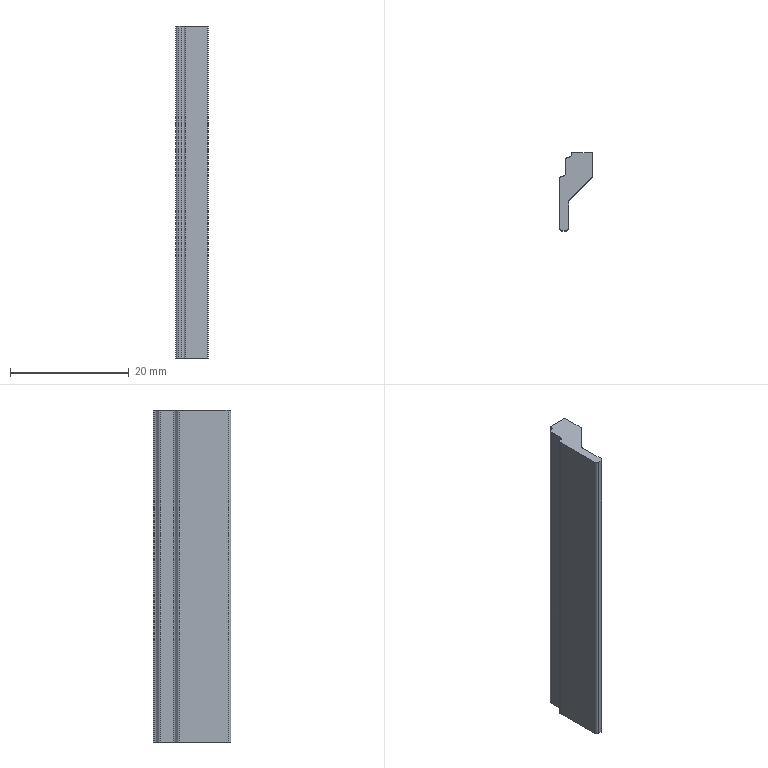Part | NX | features BREP 2 | 2 solids | 36 faces | box 5.515 x 13.15 x 56 mm | volume 4406 mm3 | plane 20 | cylinder 16 | commonest cylinder face diameters 1 x16
STEP:
#1=CARTESIAN_POINT('',(2.758,2.733,-4.));
#2=VERTEX_POINT('',#1);
#3=CARTESIAN_POINT('',(2.758,2.733,52.));
#4=VERTEX_POINT('',#3);
#5=CARTESIAN_POINT('',(2.758,2.733,0.));
#6=DIRECTION('',(0.,0.,1.));
#7=VECTOR('',#6,1000.);
#8=LINE('',#5,#7);
#9=EDGE_CURVE('',#2,#4,#8,.T.);
#10=ORIENTED_EDGE('',*,*,#9,.T.);
#11=CARTESIAN_POINT('',(2.611,2.38,52.));
#12=VERTEX_POINT('',#11);
#13=CARTESIAN_POINT('',(2.258,2.733,52.));
#14=DIRECTION('',(0.,0.,1.));
#15=DIRECTION('',(1.,0.,0.));
#16=AXIS2_PLACEMENT_3D('',#13,#14,#15);
#17=CIRCLE('',#16,0.5);
#18=EDGE_CURVE('',#12,#4,#17,.T.);
#19=ORIENTED_EDGE('',*,*,#18,.F.);
#20=CARTESIAN_POINT('',(2.611,2.38,-4.));
#21=VERTEX_POINT('',#20);
#22=CARTESIAN_POINT('',(2.611,2.38,0.));
#23=DIRECTION('',(0.,0.,1.));
#24=VECTOR('',#23,1000.);
#25=LINE('',#22,#24);
#26=EDGE_CURVE('',#21,#12,#25,.T.);
#27=ORIENTED_EDGE('',*,*,#26,.F.);
#28=CARTESIAN_POINT('',(2.258,2.733,-4.));
#29=DIRECTION('',(0.,0.,1.));
#30=DIRECTION('',(1.,0.,0.));
#31=AXIS2_PLACEMENT_3D('',#28,#29,#30);
#32=CIRCLE('',#31,0.5);
#33=EDGE_CURVE('',#21,#2,#32,.T.);
#34=ORIENTED_EDGE('',*,*,#33,.T.);
#35=EDGE_LOOP('',(#10,#19,#27,#34));
#36=FACE_BOUND('',#35,.T.);
#37=CARTESIAN_POINT('',(2.258,2.733,0.));
#38=DIRECTION('',(0.,0.,1.));
#39=DIRECTION('',(-1.,0.,0.));
#40=AXIS2_PLACEMENT_3D('',#37,#38,#39);
#41=CYLINDRICAL_SURFACE('',#40,0.5);
#42=ADVANCED_FACE('',(#36),#41,.T.);
#43=ORIENTED_EDGE('',*,*,#26,.T.);
#44=CARTESIAN_POINT('',(-1.111,-1.343,52.));
#45=VERTEX_POINT('',#44);
#46=CARTESIAN_POINT('',(2.611,2.38,52.));
#47=DIRECTION('',(0.7071,0.7071,0.));
#48=VECTOR('',#47,1000.);
#49=LINE('',#46,#48);
#50=EDGE_CURVE('',#45,#12,#49,.T.);
#51=ORIENTED_EDGE('',*,*,#50,.F.);
#52=CARTESIAN_POINT('',(-1.111,-1.343,-4.));
#53=VERTEX_POINT('',#52);
#54=CARTESIAN_POINT('',(-1.111,-1.343,0.));
#55=DIRECTION('',(0.,0.,1.));
#56=VECTOR('',#55,1000.);
#57=LINE('',#54,#56);
#58=EDGE_CURVE('',#53,#45,#57,.T.);
#59=ORIENTED_EDGE('',*,*,#58,.F.);
#60=CARTESIAN_POINT('',(2.611,2.38,-4.));
#61=DIRECTION('',(0.7071,0.7071,0.));
#62=VECTOR('',#61,1000.);
#63=LINE('',#60,#62);
#64=EDGE_CURVE('',#53,#21,#63,.T.);
#65=ORIENTED_EDGE('',*,*,#64,.T.);
#66=EDGE_LOOP('',(#43,#51,#59,#65));
#67=FACE_BOUND('',#66,.T.);
#68=CARTESIAN_POINT('',(2.611,2.38,0.));
#69=DIRECTION('',(-0.7071,0.7071,0.));
#70=DIRECTION('',(0.7071,0.7071,0.));
#71=AXIS2_PLACEMENT_3D('',#68,#69,#70);
#72=PLANE('',#71);
#73=ADVANCED_FACE('',(#67),#72,.F.);
#74=ORIENTED_EDGE('',*,*,#58,.T.);
#75=CARTESIAN_POINT('',(-1.258,-1.696,52.));
#76=VERTEX_POINT('',#75);
#77=CARTESIAN_POINT('',(-0.7577,-1.696,52.));
#78=DIRECTION('',(0.,0.,-1.));
#79=DIRECTION('',(1.,0.,0.));
#80=AXIS2_PLACEMENT_3D('',#77,#78,#79);
#81=CIRCLE('',#80,0.5);
#82=EDGE_CURVE('',#76,#45,#81,.T.);
#83=ORIENTED_EDGE('',*,*,#82,.F.);
#84=CARTESIAN_POINT('',(-1.258,-1.696,-4.));
#85=VERTEX_POINT('',#84);
#86=CARTESIAN_POINT('',(-1.258,-1.696,0.));
#87=DIRECTION('',(0.,0.,1.));
#88=VECTOR('',#87,1000.);
#89=LINE('',#86,#88);
#90=EDGE_CURVE('',#85,#76,#89,.T.);
#91=ORIENTED_EDGE('',*,*,#90,.F.);
#92=CARTESIAN_POINT('',(-0.7577,-1.696,-4.));
#93=DIRECTION('',(0.,0.,-1.));
#94=DIRECTION('',(1.,0.,0.));
#95=AXIS2_PLACEMENT_3D('',#92,#93,#94);
#96=CIRCLE('',#95,0.5);
#97=EDGE_CURVE('',#85,#53,#96,.T.);
#98=ORIENTED_EDGE('',*,*,#97,.T.);
#99=EDGE_LOOP('',(#74,#83,#91,#98));
#100=FACE_BOUND('',#99,.T.);
#101=CARTESIAN_POINT('',(-0.7577,-1.696,0.));
#102=DIRECTION('',(0.,0.,1.));
#103=DIRECTION('',(-1.,0.,0.));
#104=AXIS2_PLACEMENT_3D('',#101,#102,#103);
#105=CYLINDRICAL_SURFACE('',#104,0.5);
#106=ADVANCED_FACE('',(#100),#105,.F.);
#107=ORIENTED_EDGE('',*,*,#90,.T.);
#108=CARTESIAN_POINT('',(-1.258,-6.05,52.));
#109=VERTEX_POINT('',#108);
#110=CARTESIAN_POINT('',(-1.258,-8.572,52.));
#111=DIRECTION('',(0.,1.,0.));
#112=VECTOR('',#111,1000.);
#113=LINE('',#110,#112);
#114=EDGE_CURVE('',#109,#76,#113,.T.);
#115=ORIENTED_EDGE('',*,*,#114,.F.);
#116=CARTESIAN_POINT('',(-1.258,-6.05,-4.));
#117=VERTEX_POINT('',#116);
#118=CARTESIAN_POINT('',(-1.258,-6.05,0.));
#119=DIRECTION('',(0.,0.,1.));
#120=VECTOR('',#119,1000.);
#121=LINE('',#118,#120);
#122=EDGE_CURVE('',#117,#109,#121,.T.);
#123=ORIENTED_EDGE('',*,*,#122,.F.);
#124=CARTESIAN_POINT('',(-1.258,-8.572,-4.));
#125=DIRECTION('',(0.,1.,0.));
#126=VECTOR('',#125,1000.);
#127=LINE('',#124,#126);
#128=EDGE_CURVE('',#117,#85,#127,.T.);
#129=ORIENTED_EDGE('',*,*,#128,.T.);
#130=EDGE_LOOP('',(#107,#115,#123,#129));
#131=FACE_BOUND('',#130,.T.);
#132=CARTESIAN_POINT('',(-1.258,-1.696,0.));
#133=DIRECTION('',(-1.,0.,0.));
#134=DIRECTION('',(0.,1.,0.));
#135=AXIS2_PLACEMENT_3D('',#132,#133,#134);
#136=PLANE('',#135);
#137=ADVANCED_FACE('',(#131),#136,.F.);
#138=ORIENTED_EDGE('',*,*,#122,.T.);
#139=CARTESIAN_POINT('',(-1.758,-6.55,52.));
#140=VERTEX_POINT('',#139);
#141=CARTESIAN_POINT('',(-1.758,-6.05,52.));
#142=DIRECTION('',(0.,0.,1.));
#143=DIRECTION('',(1.,0.,0.));
#144=AXIS2_PLACEMENT_3D('',#141,#142,#143);
#145=CIRCLE('',#144,0.5);
#146=EDGE_CURVE('',#140,#109,#145,.T.);
#147=ORIENTED_EDGE('',*,*,#146,.F.);
#148=CARTESIAN_POINT('',(-1.758,-6.55,-4.));
#149=VERTEX_POINT('',#148);
#150=CARTESIAN_POINT('',(-1.758,-6.55,0.));
#151=DIRECTION('',(0.,0.,1.));
#152=VECTOR('',#151,1000.);
#153=LINE('',#150,#152);
#154=EDGE_CURVE('',#149,#140,#153,.T.);
#155=ORIENTED_EDGE('',*,*,#154,.F.);
#156=CARTESIAN_POINT('',(-1.758,-6.05,-4.));
#157=DIRECTION('',(0.,0.,1.));
#158=DIRECTION('',(1.,0.,0.));
#159=AXIS2_PLACEMENT_3D('',#156,#157,#158);
#160=CIRCLE('',#159,0.5);
#161=EDGE_CURVE('',#149,#117,#160,.T.);
#162=ORIENTED_EDGE('',*,*,#161,.T.);
#163=EDGE_LOOP('',(#138,#147,#155,#162));
#164=FACE_BOUND('',#163,.T.);
#165=CARTESIAN_POINT('',(-1.758,-6.05,0.));
#166=DIRECTION('',(0.,0.,1.));
#167=DIRECTION('',(-1.,0.,0.));
#168=AXIS2_PLACEMENT_3D('',#165,#166,#167);
#169=CYLINDRICAL_SURFACE('',#168,0.5);
#170=ADVANCED_FACE('',(#164),#169,.T.);
#171=ORIENTED_EDGE('',*,*,#154,.T.);
#172=CARTESIAN_POINT('',(-2.258,-6.55,52.));
#173=VERTEX_POINT('',#172);
#174=CARTESIAN_POINT('',(6.216,-6.55,52.));
#175=DIRECTION('',(1.,0.,0.));
#176=VECTOR('',#175,1000.);
#177=LINE('',#174,#176);
#178=EDGE_CURVE('',#173,#140,#177,.T.);
#179=ORIENTED_EDGE('',*,*,#178,.F.);
#180=CARTESIAN_POINT('',(-2.258,-6.55,-4.));
#181=VERTEX_POINT('',#180);
#182=CARTESIAN_POINT('',(-2.258,-6.55,0.));
#183=DIRECTION('',(0.,0.,1.));
#184=VECTOR('',#183,1000.);
#185=LINE('',#182,#184);
#186=EDGE_CURVE('',#181,#173,#185,.T.);
#187=ORIENTED_EDGE('',*,*,#186,.F.);
#188=CARTESIAN_POINT('',(6.216,-6.55,-4.));
#189=DIRECTION('',(1.,0.,0.));
#190=VECTOR('',#189,1000.);
#191=LINE('',#188,#190);
#192=EDGE_CURVE('',#181,#149,#191,.T.);
#193=ORIENTED_EDGE('',*,*,#192,.T.);
#194=EDGE_LOOP('',(#171,#179,#187,#193));
#195=FACE_BOUND('',#194,.T.);
#196=CARTESIAN_POINT('',(-1.758,-6.55,0.));
#197=DIRECTION('',(0.,1.,0.));
#198=DIRECTION('',(1.,0.,0.));
#199=AXIS2_PLACEMENT_3D('',#196,#197,#198);
#200=PLANE('',#199);
#201=ADVANCED_FACE('',(#195),#200,.F.);
#202=ORIENTED_EDGE('',*,*,#186,.T.);
#203=CARTESIAN_POINT('',(-2.758,-6.05,52.));
#204=VERTEX_POINT('',#203);
#205=CARTESIAN_POINT('',(-2.258,-6.05,52.));
#206=DIRECTION('',(0.,0.,1.));
#207=DIRECTION('',(1.,0.,0.));
#208=AXIS2_PLACEMENT_3D('',#205,#206,#207);
#209=CIRCLE('',#208,0.5);
#210=EDGE_CURVE('',#204,#173,#209,.T.);
#211=ORIENTED_EDGE('',*,*,#210,.F.);
#212=CARTESIAN_POINT('',(-2.758,-6.05,-4.));
#213=VERTEX_POINT('',#212);
#214=CARTESIAN_POINT('',(-2.758,-6.05,0.));
#215=DIRECTION('',(0.,0.,1.));
#216=VECTOR('',#215,1000.);
#217=LINE('',#214,#216);
#218=EDGE_CURVE('',#213,#204,#217,.T.);
#219=ORIENTED_EDGE('',*,*,#218,.F.);
#220=CARTESIAN_POINT('',(-2.258,-6.05,-4.));
#221=DIRECTION('',(0.,0.,1.));
#222=DIRECTION('',(1.,0.,0.));
#223=AXIS2_PLACEMENT_3D('',#220,#221,#222);
#224=CIRCLE('',#223,0.5);
#225=EDGE_CURVE('',#213,#181,#224,.T.);
#226=ORIENTED_EDGE('',*,*,#225,.T.);
#227=EDGE_LOOP('',(#202,#211,#219,#226));
#228=FACE_BOUND('',#227,.T.);
#229=CARTESIAN_POINT('',(-2.258,-6.05,0.));
#230=DIRECTION('',(0.,0.,1.));
#231=DIRECTION('',(-1.,0.,0.));
#232=AXIS2_PLACEMENT_3D('',#229,#230,#231);
#233=CYLINDRICAL_SURFACE('',#232,0.5);
#234=ADVANCED_FACE('',(#228),#233,.T.);
#235=ORIENTED_EDGE('',*,*,#218,.T.);
#236=CARTESIAN_POINT('',(-2.758,2.15,52.));
#237=VERTEX_POINT('',#236);
#238=CARTESIAN_POINT('',(-2.758,-8.572,52.));
#239=DIRECTION('',(0.,-1.,0.));
#240=VECTOR('',#239,1000.);
#241=LINE('',#238,#240);
#242=EDGE_CURVE('',#237,#204,#241,.T.);
#243=ORIENTED_EDGE('',*,*,#242,.F.);
#244=CARTESIAN_POINT('',(-2.758,2.15,-4.));
#245=VERTEX_POINT('',#244);
#246=CARTESIAN_POINT('',(-2.758,2.15,0.));
#247=DIRECTION('',(0.,0.,1.));
#248=VECTOR('',#247,1000.);
#249=LINE('',#246,#248);
#250=EDGE_CURVE('',#245,#237,#249,.T.);
#251=ORIENTED_EDGE('',*,*,#250,.F.);
#252=CARTESIAN_POINT('',(-2.758,-8.572,-4.));
#253=DIRECTION('',(0.,-1.,0.));
#254=VECTOR('',#253,1000.);
#255=LINE('',#252,#254);
#256=EDGE_CURVE('',#245,#213,#255,.T.);
#257=ORIENTED_EDGE('',*,*,#256,.T.);
#258=EDGE_LOOP('',(#235,#243,#251,#257));
#259=FACE_BOUND('',#258,.T.);
#260=CARTESIAN_POINT('',(-2.758,-6.05,0.));
#261=DIRECTION('',(1.,0.,0.));
#262=DIRECTION('',(0.,-1.,0.));
#263=AXIS2_PLACEMENT_3D('',#260,#261,#262);
#264=PLANE('',#263);
#265=ADVANCED_FACE('',(#259),#264,.F.);
#266=ORIENTED_EDGE('',*,*,#250,.T.);
#267=CARTESIAN_POINT('',(-2.258,2.65,52.));
#268=VERTEX_POINT('',#267);
#269=CARTESIAN_POINT('',(-2.258,2.15,52.));
#270=DIRECTION('',(0.,0.,1.));
#271=DIRECTION('',(1.,0.,0.));
#272=AXIS2_PLACEMENT_3D('',#269,#270,#271);
#273=CIRCLE('',#272,0.5);
#274=EDGE_CURVE('',#268,#237,#273,.T.);
#275=ORIENTED_EDGE('',*,*,#274,.F.);
#276=CARTESIAN_POINT('',(-2.258,2.65,-4.));
#277=VERTEX_POINT('',#276);
#278=CARTESIAN_POINT('',(-2.258,2.65,0.));
#279=DIRECTION('',(0.,0.,1.));
#280=VECTOR('',#279,1000.);
#281=LINE('',#278,#280);
#282=EDGE_CURVE('',#277,#268,#281,.T.);
#283=ORIENTED_EDGE('',*,*,#282,.F.);
#284=CARTESIAN_POINT('',(-2.258,2.15,-4.));
#285=DIRECTION('',(0.,0.,1.));
#286=DIRECTION('',(1.,0.,0.));
#287=AXIS2_PLACEMENT_3D('',#284,#285,#286);
#288=CIRCLE('',#287,0.5);
#289=EDGE_CURVE('',#277,#245,#288,.T.);
#290=ORIENTED_EDGE('',*,*,#289,.T.);
#291=EDGE_LOOP('',(#266,#275,#283,#290));
#292=FACE_BOUND('',#291,.T.);
#293=CARTESIAN_POINT('',(-2.258,2.15,0.));
#294=DIRECTION('',(0.,0.,1.));
#295=DIRECTION('',(-1.,0.,0.));
#296=AXIS2_PLACEMENT_3D('',#293,#294,#295);
#297=CYLINDRICAL_SURFACE('',#296,0.5);
#298=ADVANCED_FACE('',(#292),#297,.T.);
#299=ORIENTED_EDGE('',*,*,#282,.T.);
#300=CARTESIAN_POINT('',(-1.758,3.15,52.));
#301=VERTEX_POINT('',#300);
#302=CARTESIAN_POINT('',(-2.258,3.15,52.));
#303=DIRECTION('',(0.,0.,-1.));
#304=DIRECTION('',(1.,0.,0.));
#305=AXIS2_PLACEMENT_3D('',#302,#303,#304);
#306=CIRCLE('',#305,0.5);
#307=EDGE_CURVE('',#301,#268,#306,.T.);
#308=ORIENTED_EDGE('',*,*,#307,.F.);
#309=CARTESIAN_POINT('',(-1.758,3.15,-4.));
#310=VERTEX_POINT('',#309);
#311=CARTESIAN_POINT('',(-1.758,3.15,0.));
#312=DIRECTION('',(0.,0.,1.));
#313=VECTOR('',#312,1000.);
#314=LINE('',#311,#313);
#315=EDGE_CURVE('',#310,#301,#314,.T.);
#316=ORIENTED_EDGE('',*,*,#315,.F.);
#317=CARTESIAN_POINT('',(-2.258,3.15,-4.));
#318=DIRECTION('',(0.,0.,-1.));
#319=DIRECTION('',(1.,0.,0.));
#320=AXIS2_PLACEMENT_3D('',#317,#318,#319);
#321=CIRCLE('',#320,0.5);
#322=EDGE_CURVE('',#310,#277,#321,.T.);
#323=ORIENTED_EDGE('',*,*,#322,.T.);
#324=EDGE_LOOP('',(#299,#308,#316,#323));
#325=FACE_BOUND('',#324,.T.);
#326=CARTESIAN_POINT('',(-2.258,3.15,0.));
#327=DIRECTION('',(0.,0.,1.));
#328=DIRECTION('',(-1.,0.,0.));
#329=AXIS2_PLACEMENT_3D('',#326,#327,#328);
#330=CYLINDRICAL_SURFACE('',#329,0.5);
#331=ADVANCED_FACE('',(#325),#330,.F.);
#332=ORIENTED_EDGE('',*,*,#315,.T.);
#333=CARTESIAN_POINT('',(-1.758,5.35,52.));
#334=VERTEX_POINT('',#333);
#335=CARTESIAN_POINT('',(-1.758,-8.572,52.));
#336=DIRECTION('',(0.,-1.,0.));
#337=VECTOR('',#336,1000.);
#338=LINE('',#335,#337);
#339=EDGE_CURVE('',#334,#301,#338,.T.);
#340=ORIENTED_EDGE('',*,*,#339,.F.);
#341=CARTESIAN_POINT('',(-1.758,5.35,-4.));
#342=VERTEX_POINT('',#341);
#343=CARTESIAN_POINT('',(-1.758,5.35,0.));
#344=DIRECTION('',(0.,0.,1.));
#345=VECTOR('',#344,1000.);
#346=LINE('',#343,#345);
#347=EDGE_CURVE('',#342,#334,#346,.T.);
#348=ORIENTED_EDGE('',*,*,#347,.F.);
#349=CARTESIAN_POINT('',(-1.758,-8.572,-4.));
#350=DIRECTION('',(0.,-1.,0.));
#351=VECTOR('',#350,1000.);
#352=LINE('',#349,#351);
#353=EDGE_CURVE('',#342,#310,#352,.T.);
#354=ORIENTED_EDGE('',*,*,#353,.T.);
#355=EDGE_LOOP('',(#332,#340,#348,#354));
#356=FACE_BOUND('',#355,.T.);
#357=CARTESIAN_POINT('',(-1.758,3.15,0.));
#358=DIRECTION('',(1.,0.,0.));
#359=DIRECTION('',(0.,-1.,0.));
#360=AXIS2_PLACEMENT_3D('',#357,#358,#359);
#361=PLANE('',#360);
#362=ADVANCED_FACE('',(#356),#361,.F.);
#363=ORIENTED_EDGE('',*,*,#347,.T.);
#364=CARTESIAN_POINT('',(-1.258,5.85,52.));
#365=VERTEX_POINT('',#364);
#366=CARTESIAN_POINT('',(-1.258,5.35,52.));
#367=DIRECTION('',(0.,0.,1.));
#368=DIRECTION('',(1.,0.,0.));
#369=AXIS2_PLACEMENT_3D('',#366,#367,#368);
#370=CIRCLE('',#369,0.5);
#371=EDGE_CURVE('',#365,#334,#370,.T.);
#372=ORIENTED_EDGE('',*,*,#371,.F.);
#373=CARTESIAN_POINT('',(-1.258,5.85,-4.));
#374=VERTEX_POINT('',#373);
#375=CARTESIAN_POINT('',(-1.258,5.85,0.));
#376=DIRECTION('',(0.,0.,1.));
#377=VECTOR('',#376,1000.);
#378=LINE('',#375,#377);
#379=EDGE_CURVE('',#374,#365,#378,.T.);
#380=ORIENTED_EDGE('',*,*,#379,.F.);
#381=CARTESIAN_POINT('',(-1.258,5.35,-4.));
#382=DIRECTION('',(0.,0.,1.));
#383=DIRECTION('',(1.,0.,0.));
#384=AXIS2_PLACEMENT_3D('',#381,#382,#383);
#385=CIRCLE('',#384,0.5);
#386=EDGE_CURVE('',#374,#342,#385,.T.);
#387=ORIENTED_EDGE('',*,*,#386,.T.);
#388=EDGE_LOOP('',(#363,#372,#380,#387));
#389=FACE_BOUND('',#388,.T.);
#390=CARTESIAN_POINT('',(-1.258,5.35,0.));
#391=DIRECTION('',(0.,0.,1.));
#392=DIRECTION('',(-1.,0.,0.));
#393=AXIS2_PLACEMENT_3D('',#390,#391,#392);
#394=CYLINDRICAL_SURFACE('',#393,0.5);
#395=ADVANCED_FACE('',(#389),#394,.T.);
#396=ORIENTED_EDGE('',*,*,#379,.T.);
#397=CARTESIAN_POINT('',(-0.7577,6.35,52.));
#398=VERTEX_POINT('',#397);
#399=CARTESIAN_POINT('',(-1.258,6.35,52.));
#400=DIRECTION('',(0.,0.,-1.));
#401=DIRECTION('',(1.,0.,0.));
#402=AXIS2_PLACEMENT_3D('',#399,#400,#401);
#403=CIRCLE('',#402,0.5);
#404=EDGE_CURVE('',#398,#365,#403,.T.);
#405=ORIENTED_EDGE('',*,*,#404,.F.);
#406=CARTESIAN_POINT('',(-0.7577,6.35,-4.));
#407=VERTEX_POINT('',#406);
#408=CARTESIAN_POINT('',(-0.7577,6.35,0.));
#409=DIRECTION('',(0.,0.,1.));
#410=VECTOR('',#409,1000.);
#411=LINE('',#408,#410);
#412=EDGE_CURVE('',#407,#398,#411,.T.);
#413=ORIENTED_EDGE('',*,*,#412,.F.);
#414=CARTESIAN_POINT('',(-1.258,6.35,-4.));
#415=DIRECTION('',(0.,0.,-1.));
#416=DIRECTION('',(1.,0.,0.));
#417=AXIS2_PLACEMENT_3D('',#414,#415,#416);
#418=CIRCLE('',#417,0.5);
#419=EDGE_CURVE('',#407,#374,#418,.T.);
#420=ORIENTED_EDGE('',*,*,#419,.T.);
#421=EDGE_LOOP('',(#396,#405,#413,#420));
#422=FACE_BOUND('',#421,.T.);
#423=CARTESIAN_POINT('',(-1.258,6.35,0.));
#424=DIRECTION('',(0.,0.,1.));
#425=DIRECTION('',(-1.,0.,0.));
#426=AXIS2_PLACEMENT_3D('',#423,#424,#425);
#427=CYLINDRICAL_SURFACE('',#426,0.5);
#428=ADVANCED_FACE('',(#422),#427,.F.);
#429=ORIENTED_EDGE('',*,*,#412,.T.);
#430=CARTESIAN_POINT('',(-0.7577,6.6,52.));
#431=VERTEX_POINT('',#430);
#432=CARTESIAN_POINT('',(-0.7577,-8.572,52.));
#433=DIRECTION('',(0.,-1.,0.));
#434=VECTOR('',#433,1000.);
#435=LINE('',#432,#434);
#436=EDGE_CURVE('',#431,#398,#435,.T.);
#437=ORIENTED_EDGE('',*,*,#436,.F.);
#438=CARTESIAN_POINT('',(-0.7577,6.6,-4.));
#439=VERTEX_POINT('',#438);
#440=CARTESIAN_POINT('',(-0.7577,6.6,0.));
#441=DIRECTION('',(0.,0.,1.));
#442=VECTOR('',#441,1000.);
#443=LINE('',#440,#442);
#444=EDGE_CURVE('',#439,#431,#443,.T.);
#445=ORIENTED_EDGE('',*,*,#444,.F.);
#446=CARTESIAN_POINT('',(-0.7577,-8.572,-4.));
#447=DIRECTION('',(0.,-1.,0.));
#448=VECTOR('',#447,1000.);
#449=LINE('',#446,#448);
#450=EDGE_CURVE('',#439,#407,#449,.T.);
#451=ORIENTED_EDGE('',*,*,#450,.T.);
#452=EDGE_LOOP('',(#429,#437,#445,#451));
#453=FACE_BOUND('',#452,.T.);
#454=CARTESIAN_POINT('',(-0.7577,6.35,0.));
#455=DIRECTION('',(1.,0.,0.));
#456=DIRECTION('',(0.,-1.,0.));
#457=AXIS2_PLACEMENT_3D('',#454,#455,#456);
#458=PLANE('',#457);
#459=ADVANCED_FACE('',(#453),#458,.F.);
#460=ORIENTED_EDGE('',*,*,#444,.T.);
#461=CARTESIAN_POINT('',(2.758,6.6,52.));
#462=VERTEX_POINT('',#461);
#463=CARTESIAN_POINT('',(6.216,6.6,52.));
#464=DIRECTION('',(-1.,0.,0.));
#465=VECTOR('',#464,1000.);
#466=LINE('',#463,#465);
#467=EDGE_CURVE('',#462,#431,#466,.T.);
#468=ORIENTED_EDGE('',*,*,#467,.F.);
#469=CARTESIAN_POINT('',(2.758,6.6,-4.));
#470=VERTEX_POINT('',#469);
#471=CARTESIAN_POINT('',(2.758,6.6,0.));
#472=DIRECTION('',(0.,0.,1.));
#473=VECTOR('',#472,1000.);
#474=LINE('',#471,#473);
#475=EDGE_CURVE('',#470,#462,#474,.T.);
#476=ORIENTED_EDGE('',*,*,#475,.F.);
#477=CARTESIAN_POINT('',(6.216,6.6,-4.));
#478=DIRECTION('',(-1.,0.,0.));
#479=VECTOR('',#478,1000.);
#480=LINE('',#477,#479);
#481=EDGE_CURVE('',#470,#439,#480,.T.);
#482=ORIENTED_EDGE('',*,*,#481,.T.);
#483=EDGE_LOOP('',(#460,#468,#476,#482));
#484=FACE_BOUND('',#483,.T.);
#485=CARTESIAN_POINT('',(6.216,6.6,0.));
#486=DIRECTION('',(0.,-1.,0.));
#487=DIRECTION('',(-1.,0.,0.));
#488=AXIS2_PLACEMENT_3D('',#485,#486,#487);
#489=PLANE('',#488);
#490=ADVANCED_FACE('',(#484),#489,.F.);
#491=CARTESIAN_POINT('',(2.758,-8.572,-4.));
#492=DIRECTION('',(0.,1.,0.));
#493=VECTOR('',#492,1000.);
#494=LINE('',#491,#493);
#495=EDGE_CURVE('',#2,#470,#494,.T.);
#496=ORIENTED_EDGE('',*,*,#495,.T.);
#497=ORIENTED_EDGE('',*,*,#475,.T.);
#498=CARTESIAN_POINT('',(2.758,-8.572,52.));
#499=DIRECTION('',(0.,1.,0.));
#500=VECTOR('',#499,1000.);
#501=LINE('',#498,#500);
#502=EDGE_CURVE('',#4,#462,#501,.T.);
#503=ORIENTED_EDGE('',*,*,#502,.F.);
#504=ORIENTED_EDGE('',*,*,#9,.F.);
#505=EDGE_LOOP('',(#496,#497,#503,#504));
#506=FACE_BOUND('',#505,.T.);
#507=CARTESIAN_POINT('',(2.758,8.726,0.));
#508=DIRECTION('',(-1.,0.,0.));
#509=DIRECTION('',(0.,1.,0.));
#510=AXIS2_PLACEMENT_3D('',#507,#508,#509);
#511=PLANE('',#510);
#512=ADVANCED_FACE('',(#506),#511,.F.);
#513=ORIENTED_EDGE('',*,*,#467,.T.);
#514=ORIENTED_EDGE('',*,*,#436,.T.);
#515=ORIENTED_EDGE('',*,*,#404,.T.);
#516=ORIENTED_EDGE('',*,*,#371,.T.);
#517=ORIENTED_EDGE('',*,*,#339,.T.);
#518=ORIENTED_EDGE('',*,*,#307,.T.);
#519=ORIENTED_EDGE('',*,*,#274,.T.);
#520=ORIENTED_EDGE('',*,*,#242,.T.);
#521=ORIENTED_EDGE('',*,*,#210,.T.);
#522=ORIENTED_EDGE('',*,*,#178,.T.);
#523=ORIENTED_EDGE('',*,*,#146,.T.);
#524=ORIENTED_EDGE('',*,*,#114,.T.);
#525=ORIENTED_EDGE('',*,*,#82,.T.);
#526=ORIENTED_EDGE('',*,*,#50,.T.);
#527=ORIENTED_EDGE('',*,*,#18,.T.);
#528=ORIENTED_EDGE('',*,*,#502,.T.);
#529=EDGE_LOOP('',(#513,#514,#515,#516,#517,#518,#519,#520,#521,#522,#523,#524,#525,#526,#527,#528));
#530=FACE_BOUND('',#529,.T.);
#531=CARTESIAN_POINT('',(6.216,-8.572,52.));
#532=DIRECTION('',(0.,0.,1.));
#533=DIRECTION('',(-1.,0.,0.));
#534=AXIS2_PLACEMENT_3D('',#531,#532,#533);
#535=PLANE('',#534);
#536=ADVANCED_FACE('',(#530),#535,.T.);
#537=ORIENTED_EDGE('',*,*,#481,.F.);
#538=ORIENTED_EDGE('',*,*,#495,.F.);
#539=ORIENTED_EDGE('',*,*,#33,.F.);
#540=ORIENTED_EDGE('',*,*,#64,.F.);
#541=ORIENTED_EDGE('',*,*,#97,.F.);
#542=ORIENTED_EDGE('',*,*,#128,.F.);
#543=ORIENTED_EDGE('',*,*,#161,.F.);
#544=ORIENTED_EDGE('',*,*,#192,.F.);
#545=ORIENTED_EDGE('',*,*,#225,.F.);
#546=ORIENTED_EDGE('',*,*,#256,.F.);
#547=ORIENTED_EDGE('',*,*,#289,.F.);
#548=ORIENTED_EDGE('',*,*,#322,.F.);
#549=ORIENTED_EDGE('',*,*,#353,.F.);
#550=ORIENTED_EDGE('',*,*,#386,.F.);
#551=ORIENTED_EDGE('',*,*,#419,.F.);
#552=ORIENTED_EDGE('',*,*,#450,.F.);
#553=EDGE_LOOP('',(#537,#538,#539,#540,#541,#542,#543,#544,#545,#546,#547,#548,#549,#550,#551,#552));
#554=FACE_BOUND('',#553,.T.);
#555=CARTESIAN_POINT('',(6.216,-8.572,-4.));
#556=DIRECTION('',(0.,0.,1.));
#557=DIRECTION('',(-1.,0.,0.));
#558=AXIS2_PLACEMENT_3D('',#555,#556,#557);
#559=PLANE('',#558);
#560=ADVANCED_FACE('',(#554),#559,.F.);
#561=CLOSED_SHELL('',(#42,#73,#106,#137,#170,#201,#234,#265,#298,#331,#362,#395,#428,#459,#490,#512,#536,#560));
#562=MANIFOLD_SOLID_BREP('',#561);
#563=CARTESIAN_POINT('',(2.758,2.733,-4.));
#564=VERTEX_POINT('',#563);
#565=CARTESIAN_POINT('',(2.758,2.733,52.));
#566=VERTEX_POINT('',#565);
#567=CARTESIAN_POINT('',(2.758,2.733,0.));
#568=DIRECTION('',(0.,0.,1.));
#569=VECTOR('',#568,1000.);
#570=LINE('',#567,#569);
#571=EDGE_CURVE('',#564,#566,#570,.T.);
#572=ORIENTED_EDGE('',*,*,#571,.T.);
#573=CARTESIAN_POINT('',(2.611,2.38,52.));
#574=VERTEX_POINT('',#573);
#575=CARTESIAN_POINT('',(2.258,2.733,52.));
#576=DIRECTION('',(0.,0.,1.));
#577=DIRECTION('',(1.,0.,0.));
#578=AXIS2_PLACEMENT_3D('',#575,#576,#577);
#579=CIRCLE('',#578,0.5);
#580=EDGE_CURVE('',#574,#566,#579,.T.);
#581=ORIENTED_EDGE('',*,*,#580,.F.);
#582=CARTESIAN_POINT('',(2.611,2.38,-4.));
#583=VERTEX_POINT('',#582);
#584=CARTESIAN_POINT('',(2.611,2.38,0.));
#585=DIRECTION('',(0.,0.,1.));
#586=VECTOR('',#585,1000.);
#587=LINE('',#584,#586);
#588=EDGE_CURVE('',#583,#574,#587,.T.);
#589=ORIENTED_EDGE('',*,*,#588,.F.);
#590=CARTESIAN_POINT('',(2.258,2.733,-4.));
#591=DIRECTION('',(0.,0.,1.));
#592=DIRECTION('',(1.,0.,0.));
#593=AXIS2_PLACEMENT_3D('',#590,#591,#592);
#594=CIRCLE('',#593,0.5);
#595=EDGE_CURVE('',#583,#564,#594,.T.);
#596=ORIENTED_EDGE('',*,*,#595,.T.);
#597=EDGE_LOOP('',(#572,#581,#589,#596));
#598=FACE_BOUND('',#597,.T.);
#599=CARTESIAN_POINT('',(2.258,2.733,0.));
#600=DIRECTION('',(0.,0.,1.));
#601=DIRECTION('',(-1.,0.,0.));
#602=AXIS2_PLACEMENT_3D('',#599,#600,#601);
#603=CYLINDRICAL_SURFACE('',#602,0.5);
#604=ADVANCED_FACE('',(#598),#603,.T.);
#605=ORIENTED_EDGE('',*,*,#588,.T.);
#606=CARTESIAN_POINT('',(-1.111,-1.343,52.));
#607=VERTEX_POINT('',#606);
#608=CARTESIAN_POINT('',(2.611,2.38,52.));
#609=DIRECTION('',(0.7071,0.7071,0.));
#610=VECTOR('',#609,1000.);
#611=LINE('',#608,#610);
#612=EDGE_CURVE('',#607,#574,#611,.T.);
#613=ORIENTED_EDGE('',*,*,#612,.F.);
#614=CARTESIAN_POINT('',(-1.111,-1.343,-4.));
#615=VERTEX_POINT('',#614);
#616=CARTESIAN_POINT('',(-1.111,-1.343,0.));
#617=DIRECTION('',(0.,0.,1.));
#618=VECTOR('',#617,1000.);
#619=LINE('',#616,#618);
#620=EDGE_CURVE('',#615,#607,#619,.T.);
#621=ORIENTED_EDGE('',*,*,#620,.F.);
#622=CARTESIAN_POINT('',(2.611,2.38,-4.));
#623=DIRECTION('',(0.7071,0.7071,0.));
#624=VECTOR('',#623,1000.);
#625=LINE('',#622,#624);
#626=EDGE_CURVE('',#615,#583,#625,.T.);
#627=ORIENTED_EDGE('',*,*,#626,.T.);
#628=EDGE_LOOP('',(#605,#613,#621,#627));
#629=FACE_BOUND('',#628,.T.);
#630=CARTESIAN_POINT('',(2.611,2.38,0.));
#631=DIRECTION('',(-0.7071,0.7071,0.));
#632=DIRECTION('',(0.7071,0.7071,0.));
#633=AXIS2_PLACEMENT_3D('',#630,#631,#632);
#634=PLANE('',#633);
#635=ADVANCED_FACE('',(#629),#634,.F.);
#636=ORIENTED_EDGE('',*,*,#620,.T.);
#637=CARTESIAN_POINT('',(-1.258,-1.696,52.));
#638=VERTEX_POINT('',#637);
#639=CARTESIAN_POINT('',(-0.7577,-1.696,52.));
#640=DIRECTION('',(0.,0.,-1.));
#641=DIRECTION('',(1.,0.,0.));
#642=AXIS2_PLACEMENT_3D('',#639,#640,#641);
#643=CIRCLE('',#642,0.5);
#644=EDGE_CURVE('',#638,#607,#643,.T.);
#645=ORIENTED_EDGE('',*,*,#644,.F.);
#646=CARTESIAN_POINT('',(-1.258,-1.696,-4.));
#647=VERTEX_POINT('',#646);
#648=CARTESIAN_POINT('',(-1.258,-1.696,0.));
#649=DIRECTION('',(0.,0.,1.));
#650=VECTOR('',#649,1000.);
#651=LINE('',#648,#650);
#652=EDGE_CURVE('',#647,#638,#651,.T.);
#653=ORIENTED_EDGE('',*,*,#652,.F.);
#654=CARTESIAN_POINT('',(-0.7577,-1.696,-4.));
#655=DIRECTION('',(0.,0.,-1.));
#656=DIRECTION('',(1.,0.,0.));
#657=AXIS2_PLACEMENT_3D('',#654,#655,#656);
#658=CIRCLE('',#657,0.5);
#659=EDGE_CURVE('',#647,#615,#658,.T.);
#660=ORIENTED_EDGE('',*,*,#659,.T.);
#661=EDGE_LOOP('',(#636,#645,#653,#660));
#662=FACE_BOUND('',#661,.T.);
#663=CARTESIAN_POINT('',(-0.7577,-1.696,0.));
#664=DIRECTION('',(0.,0.,1.));
#665=DIRECTION('',(-1.,0.,0.));
#666=AXIS2_PLACEMENT_3D('',#663,#664,#665);
#667=CYLINDRICAL_SURFACE('',#666,0.5);
#668=ADVANCED_FACE('',(#662),#667,.F.);
#669=ORIENTED_EDGE('',*,*,#652,.T.);
#670=CARTESIAN_POINT('',(-1.258,-6.05,52.));
#671=VERTEX_POINT('',#670);
#672=CARTESIAN_POINT('',(-1.258,-8.572,52.));
#673=DIRECTION('',(0.,1.,0.));
#674=VECTOR('',#673,1000.);
#675=LINE('',#672,#674);
#676=EDGE_CURVE('',#671,#638,#675,.T.);
#677=ORIENTED_EDGE('',*,*,#676,.F.);
#678=CARTESIAN_POINT('',(-1.258,-6.05,-4.));
#679=VERTEX_POINT('',#678);
#680=CARTESIAN_POINT('',(-1.258,-6.05,0.));
#681=DIRECTION('',(0.,0.,1.));
#682=VECTOR('',#681,1000.);
#683=LINE('',#680,#682);
#684=EDGE_CURVE('',#679,#671,#683,.T.);
#685=ORIENTED_EDGE('',*,*,#684,.F.);
#686=CARTESIAN_POINT('',(-1.258,-8.572,-4.));
#687=DIRECTION('',(0.,1.,0.));
#688=VECTOR('',#687,1000.);
#689=LINE('',#686,#688);
#690=EDGE_CURVE('',#679,#647,#689,.T.);
#691=ORIENTED_EDGE('',*,*,#690,.T.);
#692=EDGE_LOOP('',(#669,#677,#685,#691));
#693=FACE_BOUND('',#692,.T.);
#694=CARTESIAN_POINT('',(-1.258,-1.696,0.));
#695=DIRECTION('',(-1.,0.,0.));
#696=DIRECTION('',(0.,1.,0.));
#697=AXIS2_PLACEMENT_3D('',#694,#695,#696);
#698=PLANE('',#697);
#699=ADVANCED_FACE('',(#693),#698,.F.);
#700=ORIENTED_EDGE('',*,*,#684,.T.);
#701=CARTESIAN_POINT('',(-1.758,-6.55,52.));
#702=VERTEX_POINT('',#701);
#703=CARTESIAN_POINT('',(-1.758,-6.05,52.));
#704=DIRECTION('',(0.,0.,1.));
#705=DIRECTION('',(1.,0.,0.));
#706=AXIS2_PLACEMENT_3D('',#703,#704,#705);
#707=CIRCLE('',#706,0.5);
#708=EDGE_CURVE('',#702,#671,#707,.T.);
#709=ORIENTED_EDGE('',*,*,#708,.F.);
#710=CARTESIAN_POINT('',(-1.758,-6.55,-4.));
#711=VERTEX_POINT('',#710);
#712=CARTESIAN_POINT('',(-1.758,-6.55,0.));
#713=DIRECTION('',(0.,0.,1.));
#714=VECTOR('',#713,1000.);
#715=LINE('',#712,#714);
#716=EDGE_CURVE('',#711,#702,#715,.T.);
#717=ORIENTED_EDGE('',*,*,#716,.F.);
#718=CARTESIAN_POINT('',(-1.758,-6.05,-4.));
#719=DIRECTION('',(0.,0.,1.));
#720=DIRECTION('',(1.,0.,0.));
#721=AXIS2_PLACEMENT_3D('',#718,#719,#720);
#722=CIRCLE('',#721,0.5);
#723=EDGE_CURVE('',#711,#679,#722,.T.);
#724=ORIENTED_EDGE('',*,*,#723,.T.);
#725=EDGE_LOOP('',(#700,#709,#717,#724));
#726=FACE_BOUND('',#725,.T.);
#727=CARTESIAN_POINT('',(-1.758,-6.05,0.));
#728=DIRECTION('',(0.,0.,1.));
#729=DIRECTION('',(-1.,0.,0.));
#730=AXIS2_PLACEMENT_3D('',#727,#728,#729);
#731=CYLINDRICAL_SURFACE('',#730,0.5);
#732=ADVANCED_FACE('',(#726),#731,.T.);
#733=ORIENTED_EDGE('',*,*,#716,.T.);
#734=CARTESIAN_POINT('',(-2.258,-6.55,52.));
#735=VERTEX_POINT('',#734);
#736=CARTESIAN_POINT('',(6.216,-6.55,52.));
#737=DIRECTION('',(1.,0.,0.));
#738=VECTOR('',#737,1000.);
#739=LINE('',#736,#738);
#740=EDGE_CURVE('',#735,#702,#739,.T.);
#741=ORIENTED_EDGE('',*,*,#740,.F.);
#742=CARTESIAN_POINT('',(-2.258,-6.55,-4.));
#743=VERTEX_POINT('',#742);
#744=CARTESIAN_POINT('',(-2.258,-6.55,0.));
#745=DIRECTION('',(0.,0.,1.));
#746=VECTOR('',#745,1000.);
#747=LINE('',#744,#746);
#748=EDGE_CURVE('',#743,#735,#747,.T.);
#749=ORIENTED_EDGE('',*,*,#748,.F.);
#750=CARTESIAN_POINT('',(6.216,-6.55,-4.));
#751=DIRECTION('',(1.,0.,0.));
#752=VECTOR('',#751,1000.);
#753=LINE('',#750,#752);
#754=EDGE_CURVE('',#743,#711,#753,.T.);
#755=ORIENTED_EDGE('',*,*,#754,.T.);
#756=EDGE_LOOP('',(#733,#741,#749,#755));
#757=FACE_BOUND('',#756,.T.);
#758=CARTESIAN_POINT('',(-1.758,-6.55,0.));
#759=DIRECTION('',(0.,1.,0.));
#760=DIRECTION('',(1.,0.,0.));
#761=AXIS2_PLACEMENT_3D('',#758,#759,#760);
#762=PLANE('',#761);
#763=ADVANCED_FACE('',(#757),#762,.F.);
#764=ORIENTED_EDGE('',*,*,#748,.T.);
#765=CARTESIAN_POINT('',(-2.758,-6.05,52.));
#766=VERTEX_POINT('',#765);
#767=CARTESIAN_POINT('',(-2.258,-6.05,52.));
#768=DIRECTION('',(0.,0.,1.));
#769=DIRECTION('',(1.,0.,0.));
#770=AXIS2_PLACEMENT_3D('',#767,#768,#769);
#771=CIRCLE('',#770,0.5);
#772=EDGE_CURVE('',#766,#735,#771,.T.);
#773=ORIENTED_EDGE('',*,*,#772,.F.);
#774=CARTESIAN_POINT('',(-2.758,-6.05,-4.));
#775=VERTEX_POINT('',#774);
#776=CARTESIAN_POINT('',(-2.758,-6.05,0.));
#777=DIRECTION('',(0.,0.,1.));
#778=VECTOR('',#777,1000.);
#779=LINE('',#776,#778);
#780=EDGE_CURVE('',#775,#766,#779,.T.);
#781=ORIENTED_EDGE('',*,*,#780,.F.);
#782=CARTESIAN_POINT('',(-2.258,-6.05,-4.));
#783=DIRECTION('',(0.,0.,1.));
#784=DIRECTION('',(1.,0.,0.));
#785=AXIS2_PLACEMENT_3D('',#782,#783,#784);
#786=CIRCLE('',#785,0.5);
#787=EDGE_CURVE('',#775,#743,#786,.T.);
#788=ORIENTED_EDGE('',*,*,#787,.T.);
#789=EDGE_LOOP('',(#764,#773,#781,#788));
#790=FACE_BOUND('',#789,.T.);
#791=CARTESIAN_POINT('',(-2.258,-6.05,0.));
#792=DIRECTION('',(0.,0.,1.));
#793=DIRECTION('',(-1.,0.,0.));
#794=AXIS2_PLACEMENT_3D('',#791,#792,#793);
#795=CYLINDRICAL_SURFACE('',#794,0.5);
#796=ADVANCED_FACE('',(#790),#795,.T.);
#797=ORIENTED_EDGE('',*,*,#780,.T.);
#798=CARTESIAN_POINT('',(-2.758,2.15,52.));
#799=VERTEX_POINT('',#798);
#800=CARTESIAN_POINT('',(-2.758,-8.572,52.));
#801=DIRECTION('',(0.,-1.,0.));
#802=VECTOR('',#801,1000.);
#803=LINE('',#800,#802);
#804=EDGE_CURVE('',#799,#766,#803,.T.);
#805=ORIENTED_EDGE('',*,*,#804,.F.);
#806=CARTESIAN_POINT('',(-2.758,2.15,-4.));
#807=VERTEX_POINT('',#806);
#808=CARTESIAN_POINT('',(-2.758,2.15,0.));
#809=DIRECTION('',(0.,0.,1.));
#810=VECTOR('',#809,1000.);
#811=LINE('',#808,#810);
#812=EDGE_CURVE('',#807,#799,#811,.T.);
#813=ORIENTED_EDGE('',*,*,#812,.F.);
#814=CARTESIAN_POINT('',(-2.758,-8.572,-4.));
#815=DIRECTION('',(0.,-1.,0.));
#816=VECTOR('',#815,1000.);
#817=LINE('',#814,#816);
#818=EDGE_CURVE('',#807,#775,#817,.T.);
#819=ORIENTED_EDGE('',*,*,#818,.T.);
#820=EDGE_LOOP('',(#797,#805,#813,#819));
#821=FACE_BOUND('',#820,.T.);
#822=CARTESIAN_POINT('',(-2.758,-6.05,0.));
#823=DIRECTION('',(1.,0.,0.));
#824=DIRECTION('',(0.,-1.,0.));
#825=AXIS2_PLACEMENT_3D('',#822,#823,#824);
#826=PLANE('',#825);
#827=ADVANCED_FACE('',(#821),#826,.F.);
#828=ORIENTED_EDGE('',*,*,#812,.T.);
#829=CARTESIAN_POINT('',(-2.258,2.65,52.));
#830=VERTEX_POINT('',#829);
#831=CARTESIAN_POINT('',(-2.258,2.15,52.));
#832=DIRECTION('',(0.,0.,1.));
#833=DIRECTION('',(1.,0.,0.));
#834=AXIS2_PLACEMENT_3D('',#831,#832,#833);
#835=CIRCLE('',#834,0.5);
#836=EDGE_CURVE('',#830,#799,#835,.T.);
#837=ORIENTED_EDGE('',*,*,#836,.F.);
#838=CARTESIAN_POINT('',(-2.258,2.65,-4.));
#839=VERTEX_POINT('',#838);
#840=CARTESIAN_POINT('',(-2.258,2.65,0.));
#841=DIRECTION('',(0.,0.,1.));
#842=VECTOR('',#841,1000.);
#843=LINE('',#840,#842);
#844=EDGE_CURVE('',#839,#830,#843,.T.);
#845=ORIENTED_EDGE('',*,*,#844,.F.);
#846=CARTESIAN_POINT('',(-2.258,2.15,-4.));
#847=DIRECTION('',(0.,0.,1.));
#848=DIRECTION('',(1.,0.,0.));
#849=AXIS2_PLACEMENT_3D('',#846,#847,#848);
#850=CIRCLE('',#849,0.5);
#851=EDGE_CURVE('',#839,#807,#850,.T.);
#852=ORIENTED_EDGE('',*,*,#851,.T.);
#853=EDGE_LOOP('',(#828,#837,#845,#852));
#854=FACE_BOUND('',#853,.T.);
#855=CARTESIAN_POINT('',(-2.258,2.15,0.));
#856=DIRECTION('',(0.,0.,1.));
#857=DIRECTION('',(-1.,0.,0.));
#858=AXIS2_PLACEMENT_3D('',#855,#856,#857);
#859=CYLINDRICAL_SURFACE('',#858,0.5);
#860=ADVANCED_FACE('',(#854),#859,.T.);
#861=ORIENTED_EDGE('',*,*,#844,.T.);
#862=CARTESIAN_POINT('',(-1.758,3.15,52.));
#863=VERTEX_POINT('',#862);
#864=CARTESIAN_POINT('',(-2.258,3.15,52.));
#865=DIRECTION('',(0.,0.,-1.));
#866=DIRECTION('',(1.,0.,0.));
#867=AXIS2_PLACEMENT_3D('',#864,#865,#866);
#868=CIRCLE('',#867,0.5);
#869=EDGE_CURVE('',#863,#830,#868,.T.);
#870=ORIENTED_EDGE('',*,*,#869,.F.);
#871=CARTESIAN_POINT('',(-1.758,3.15,-4.));
#872=VERTEX_POINT('',#871);
#873=CARTESIAN_POINT('',(-1.758,3.15,0.));
#874=DIRECTION('',(0.,0.,1.));
#875=VECTOR('',#874,1000.);
#876=LINE('',#873,#875);
#877=EDGE_CURVE('',#872,#863,#876,.T.);
#878=ORIENTED_EDGE('',*,*,#877,.F.);
#879=CARTESIAN_POINT('',(-2.258,3.15,-4.));
#880=DIRECTION('',(0.,0.,-1.));
#881=DIRECTION('',(1.,0.,0.));
#882=AXIS2_PLACEMENT_3D('',#879,#880,#881);
#883=CIRCLE('',#882,0.5);
#884=EDGE_CURVE('',#872,#839,#883,.T.);
#885=ORIENTED_EDGE('',*,*,#884,.T.);
#886=EDGE_LOOP('',(#861,#870,#878,#885));
#887=FACE_BOUND('',#886,.T.);
#888=CARTESIAN_POINT('',(-2.258,3.15,0.));
#889=DIRECTION('',(0.,0.,1.));
#890=DIRECTION('',(-1.,0.,0.));
#891=AXIS2_PLACEMENT_3D('',#888,#889,#890);
#892=CYLINDRICAL_SURFACE('',#891,0.5);
#893=ADVANCED_FACE('',(#887),#892,.F.);
#894=ORIENTED_EDGE('',*,*,#877,.T.);
#895=CARTESIAN_POINT('',(-1.758,5.35,52.));
#896=VERTEX_POINT('',#895);
#897=CARTESIAN_POINT('',(-1.758,-8.572,52.));
#898=DIRECTION('',(0.,-1.,0.));
#899=VECTOR('',#898,1000.);
#900=LINE('',#897,#899);
#901=EDGE_CURVE('',#896,#863,#900,.T.);
#902=ORIENTED_EDGE('',*,*,#901,.F.);
#903=CARTESIAN_POINT('',(-1.758,5.35,-4.));
#904=VERTEX_POINT('',#903);
#905=CARTESIAN_POINT('',(-1.758,5.35,0.));
#906=DIRECTION('',(0.,0.,1.));
#907=VECTOR('',#906,1000.);
#908=LINE('',#905,#907);
#909=EDGE_CURVE('',#904,#896,#908,.T.);
#910=ORIENTED_EDGE('',*,*,#909,.F.);
#911=CARTESIAN_POINT('',(-1.758,-8.572,-4.));
#912=DIRECTION('',(0.,-1.,0.));
#913=VECTOR('',#912,1000.);
#914=LINE('',#911,#913);
#915=EDGE_CURVE('',#904,#872,#914,.T.);
#916=ORIENTED_EDGE('',*,*,#915,.T.);
#917=EDGE_LOOP('',(#894,#902,#910,#916));
#918=FACE_BOUND('',#917,.T.);
#919=CARTESIAN_POINT('',(-1.758,3.15,0.));
#920=DIRECTION('',(1.,0.,0.));
#921=DIRECTION('',(0.,-1.,0.));
#922=AXIS2_PLACEMENT_3D('',#919,#920,#921);
#923=PLANE('',#922);
#924=ADVANCED_FACE('',(#918),#923,.F.);
#925=ORIENTED_EDGE('',*,*,#909,.T.);
#926=CARTESIAN_POINT('',(-1.258,5.85,52.));
#927=VERTEX_POINT('',#926);
#928=CARTESIAN_POINT('',(-1.258,5.35,52.));
#929=DIRECTION('',(0.,0.,1.));
#930=DIRECTION('',(1.,0.,0.));
#931=AXIS2_PLACEMENT_3D('',#928,#929,#930);
#932=CIRCLE('',#931,0.5);
#933=EDGE_CURVE('',#927,#896,#932,.T.);
#934=ORIENTED_EDGE('',*,*,#933,.F.);
#935=CARTESIAN_POINT('',(-1.258,5.85,-4.));
#936=VERTEX_POINT('',#935);
#937=CARTESIAN_POINT('',(-1.258,5.85,0.));
#938=DIRECTION('',(0.,0.,1.));
#939=VECTOR('',#938,1000.);
#940=LINE('',#937,#939);
#941=EDGE_CURVE('',#936,#927,#940,.T.);
#942=ORIENTED_EDGE('',*,*,#941,.F.);
#943=CARTESIAN_POINT('',(-1.258,5.35,-4.));
#944=DIRECTION('',(0.,0.,1.));
#945=DIRECTION('',(1.,0.,0.));
#946=AXIS2_PLACEMENT_3D('',#943,#944,#945);
#947=CIRCLE('',#946,0.5);
#948=EDGE_CURVE('',#936,#904,#947,.T.);
#949=ORIENTED_EDGE('',*,*,#948,.T.);
#950=EDGE_LOOP('',(#925,#934,#942,#949));
#951=FACE_BOUND('',#950,.T.);
#952=CARTESIAN_POINT('',(-1.258,5.35,0.));
#953=DIRECTION('',(0.,0.,1.));
#954=DIRECTION('',(-1.,0.,0.));
#955=AXIS2_PLACEMENT_3D('',#952,#953,#954);
#956=CYLINDRICAL_SURFACE('',#955,0.5);
#957=ADVANCED_FACE('',(#951),#956,.T.);
#958=ORIENTED_EDGE('',*,*,#941,.T.);
#959=CARTESIAN_POINT('',(-0.7577,6.35,52.));
#960=VERTEX_POINT('',#959);
#961=CARTESIAN_POINT('',(-1.258,6.35,52.));
#962=DIRECTION('',(0.,0.,-1.));
#963=DIRECTION('',(1.,0.,0.));
#964=AXIS2_PLACEMENT_3D('',#961,#962,#963);
#965=CIRCLE('',#964,0.5);
#966=EDGE_CURVE('',#960,#927,#965,.T.);
#967=ORIENTED_EDGE('',*,*,#966,.F.);
#968=CARTESIAN_POINT('',(-0.7577,6.35,-4.));
#969=VERTEX_POINT('',#968);
#970=CARTESIAN_POINT('',(-0.7577,6.35,0.));
#971=DIRECTION('',(0.,0.,1.));
#972=VECTOR('',#971,1000.);
#973=LINE('',#970,#972);
#974=EDGE_CURVE('',#969,#960,#973,.T.);
#975=ORIENTED_EDGE('',*,*,#974,.F.);
#976=CARTESIAN_POINT('',(-1.258,6.35,-4.));
#977=DIRECTION('',(0.,0.,-1.));
#978=DIRECTION('',(1.,0.,0.));
#979=AXIS2_PLACEMENT_3D('',#976,#977,#978);
#980=CIRCLE('',#979,0.5);
#981=EDGE_CURVE('',#969,#936,#980,.T.);
#982=ORIENTED_EDGE('',*,*,#981,.T.);
#983=EDGE_LOOP('',(#958,#967,#975,#982));
#984=FACE_BOUND('',#983,.T.);
#985=CARTESIAN_POINT('',(-1.258,6.35,0.));
#986=DIRECTION('',(0.,0.,1.));
#987=DIRECTION('',(-1.,0.,0.));
#988=AXIS2_PLACEMENT_3D('',#985,#986,#987);
#989=CYLINDRICAL_SURFACE('',#988,0.5);
#990=ADVANCED_FACE('',(#984),#989,.F.);
#991=ORIENTED_EDGE('',*,*,#974,.T.);
#992=CARTESIAN_POINT('',(-0.7577,6.6,52.));
#993=VERTEX_POINT('',#992);
#994=CARTESIAN_POINT('',(-0.7577,-8.572,52.));
#995=DIRECTION('',(0.,-1.,0.));
#996=VECTOR('',#995,1000.);
#997=LINE('',#994,#996);
#998=EDGE_CURVE('',#993,#960,#997,.T.);
#999=ORIENTED_EDGE('',*,*,#998,.F.);
#1000=CARTESIAN_POINT('',(-0.7577,6.6,-4.));
#1001=VERTEX_POINT('',#1000);
#1002=CARTESIAN_POINT('',(-0.7577,6.6,0.));
#1003=DIRECTION('',(0.,0.,1.));
#1004=VECTOR('',#1003,1000.);
#1005=LINE('',#1002,#1004);
#1006=EDGE_CURVE('',#1001,#993,#1005,.T.);
#1007=ORIENTED_EDGE('',*,*,#1006,.F.);
#1008=CARTESIAN_POINT('',(-0.7577,-8.572,-4.));
#1009=DIRECTION('',(0.,-1.,0.));
#1010=VECTOR('',#1009,1000.);
#1011=LINE('',#1008,#1010);
#1012=EDGE_CURVE('',#1001,#969,#1011,.T.);
#1013=ORIENTED_EDGE('',*,*,#1012,.T.);
#1014=EDGE_LOOP('',(#991,#999,#1007,#1013));
#1015=FACE_BOUND('',#1014,.T.);
#1016=CARTESIAN_POINT('',(-0.7577,6.35,0.));
#1017=DIRECTION('',(1.,0.,0.));
#1018=DIRECTION('',(0.,-1.,0.));
#1019=AXIS2_PLACEMENT_3D('',#1016,#1017,#1018);
#1020=PLANE('',#1019);
#1021=ADVANCED_FACE('',(#1015),#1020,.F.);
#1022=ORIENTED_EDGE('',*,*,#1006,.T.);
#1023=CARTESIAN_POINT('',(2.758,6.6,52.));
#1024=VERTEX_POINT('',#1023);
#1025=CARTESIAN_POINT('',(6.216,6.6,52.));
#1026=DIRECTION('',(-1.,0.,0.));
#1027=VECTOR('',#1026,1000.);
#1028=LINE('',#1025,#1027);
#1029=EDGE_CURVE('',#1024,#993,#1028,.T.);
#1030=ORIENTED_EDGE('',*,*,#1029,.F.);
#1031=CARTESIAN_POINT('',(2.758,6.6,-4.));
#1032=VERTEX_POINT('',#1031);
#1033=CARTESIAN_POINT('',(2.758,6.6,0.));
#1034=DIRECTION('',(0.,0.,1.));
#1035=VECTOR('',#1034,1000.);
#1036=LINE('',#1033,#1035);
#1037=EDGE_CURVE('',#1032,#1024,#1036,.T.);
#1038=ORIENTED_EDGE('',*,*,#1037,.F.);
#1039=CARTESIAN_POINT('',(6.216,6.6,-4.));
#1040=DIRECTION('',(-1.,0.,0.));
#1041=VECTOR('',#1040,1000.);
#1042=LINE('',#1039,#1041);
#1043=EDGE_CURVE('',#1032,#1001,#1042,.T.);
#1044=ORIENTED_EDGE('',*,*,#1043,.T.);
#1045=EDGE_LOOP('',(#1022,#1030,#1038,#1044));
#1046=FACE_BOUND('',#1045,.T.);
#1047=CARTESIAN_POINT('',(6.216,6.6,0.));
#1048=DIRECTION('',(0.,-1.,0.));
#1049=DIRECTION('',(-1.,0.,0.));
#1050=AXIS2_PLACEMENT_3D('',#1047,#1048,#1049);
#1051=PLANE('',#1050);
#1052=ADVANCED_FACE('',(#1046),#1051,.F.);
#1053=CARTESIAN_POINT('',(2.758,-8.572,-4.));
#1054=DIRECTION('',(0.,1.,0.));
#1055=VECTOR('',#1054,1000.);
#1056=LINE('',#1053,#1055);
#1057=EDGE_CURVE('',#564,#1032,#1056,.T.);
#1058=ORIENTED_EDGE('',*,*,#1057,.T.);
#1059=ORIENTED_EDGE('',*,*,#1037,.T.);
#1060=CARTESIAN_POINT('',(2.758,-8.572,52.));
#1061=DIRECTION('',(0.,1.,0.));
#1062=VECTOR('',#1061,1000.);
#1063=LINE('',#1060,#1062);
#1064=EDGE_CURVE('',#566,#1024,#1063,.T.);
#1065=ORIENTED_EDGE('',*,*,#1064,.F.);
#1066=ORIENTED_EDGE('',*,*,#571,.F.);
#1067=EDGE_LOOP('',(#1058,#1059,#1065,#1066));
#1068=FACE_BOUND('',#1067,.T.);
#1069=CARTESIAN_POINT('',(2.758,8.726,0.));
#1070=DIRECTION('',(-1.,0.,0.));
#1071=DIRECTION('',(0.,1.,0.));
#1072=AXIS2_PLACEMENT_3D('',#1069,#1070,#1071);
#1073=PLANE('',#1072);
#1074=ADVANCED_FACE('',(#1068),#1073,.F.);
#1075=ORIENTED_EDGE('',*,*,#1029,.T.);
#1076=ORIENTED_EDGE('',*,*,#998,.T.);
#1077=ORIENTED_EDGE('',*,*,#966,.T.);
#1078=ORIENTED_EDGE('',*,*,#933,.T.);
#1079=ORIENTED_EDGE('',*,*,#901,.T.);
#1080=ORIENTED_EDGE('',*,*,#869,.T.);
#1081=ORIENTED_EDGE('',*,*,#836,.T.);
#1082=ORIENTED_EDGE('',*,*,#804,.T.);
#1083=ORIENTED_EDGE('',*,*,#772,.T.);
#1084=ORIENTED_EDGE('',*,*,#740,.T.);
#1085=ORIENTED_EDGE('',*,*,#708,.T.);
#1086=ORIENTED_EDGE('',*,*,#676,.T.);
#1087=ORIENTED_EDGE('',*,*,#644,.T.);
#1088=ORIENTED_EDGE('',*,*,#612,.T.);
#1089=ORIENTED_EDGE('',*,*,#580,.T.);
#1090=ORIENTED_EDGE('',*,*,#1064,.T.);
#1091=EDGE_LOOP('',(#1075,#1076,#1077,#1078,#1079,#1080,#1081,#1082,#1083,#1084,#1085,#1086,#1087,#1088,#1089,#1090));
#1092=FACE_BOUND('',#1091,.T.);
#1093=CARTESIAN_POINT('',(6.216,-8.572,52.));
#1094=DIRECTION('',(0.,0.,1.));
#1095=DIRECTION('',(-1.,0.,0.));
#1096=AXIS2_PLACEMENT_3D('',#1093,#1094,#1095);
#1097=PLANE('',#1096);
#1098=ADVANCED_FACE('',(#1092),#1097,.T.);
#1099=ORIENTED_EDGE('',*,*,#1043,.F.);
#1100=ORIENTED_EDGE('',*,*,#1057,.F.);
#1101=ORIENTED_EDGE('',*,*,#595,.F.);
#1102=ORIENTED_EDGE('',*,*,#626,.F.);
#1103=ORIENTED_EDGE('',*,*,#659,.F.);
#1104=ORIENTED_EDGE('',*,*,#690,.F.);
#1105=ORIENTED_EDGE('',*,*,#723,.F.);
#1106=ORIENTED_EDGE('',*,*,#754,.F.);
#1107=ORIENTED_EDGE('',*,*,#787,.F.);
#1108=ORIENTED_EDGE('',*,*,#818,.F.);
#1109=ORIENTED_EDGE('',*,*,#851,.F.);
#1110=ORIENTED_EDGE('',*,*,#884,.F.);
#1111=ORIENTED_EDGE('',*,*,#915,.F.);
#1112=ORIENTED_EDGE('',*,*,#948,.F.);
#1113=ORIENTED_EDGE('',*,*,#981,.F.);
#1114=ORIENTED_EDGE('',*,*,#1012,.F.);
#1115=EDGE_LOOP('',(#1099,#1100,#1101,#1102,#1103,#1104,#1105,#1106,#1107,#1108,#1109,#1110,#1111,#1112,#1113,#1114));
#1116=FACE_BOUND('',#1115,.T.);
#1117=CARTESIAN_POINT('',(6.216,-8.572,-4.));
#1118=DIRECTION('',(0.,0.,1.));
#1119=DIRECTION('',(-1.,0.,0.));
#1120=AXIS2_PLACEMENT_3D('',#1117,#1118,#1119);
#1121=PLANE('',#1120);
#1122=ADVANCED_FACE('',(#1116),#1121,.F.);
#1123=CLOSED_SHELL('',(#604,#635,#668,#699,#732,#763,#796,#827,#860,#893,#924,#957,#990,#1021,#1052,#1074,#1098,#1122));
#1124=MANIFOLD_SOLID_BREP('',#1123);
#1125=(LENGTH_UNIT()NAMED_UNIT(*)SI_UNIT(.MILLI.,.METRE.));
#1126=UNCERTAINTY_MEASURE_WITH_UNIT(LENGTH_MEASURE(0.00001),#1125,'','');
#1127=(NAMED_UNIT(*)PLANE_ANGLE_UNIT()SI_UNIT($,.RADIAN.));
#1128=(NAMED_UNIT(*)SI_UNIT($,.STERADIAN.)SOLID_ANGLE_UNIT());
#1129=(GEOMETRIC_REPRESENTATION_CONTEXT(3)GLOBAL_UNCERTAINTY_ASSIGNED_CONTEXT((#1126))GLOBAL_UNIT_ASSIGNED_CONTEXT((#1125,#1127,#1128))REPRESENTATION_CONTEXT('',''));
#1130=ADVANCED_BREP_SHAPE_REPRESENTATION('',(#562,#1124),#1129);